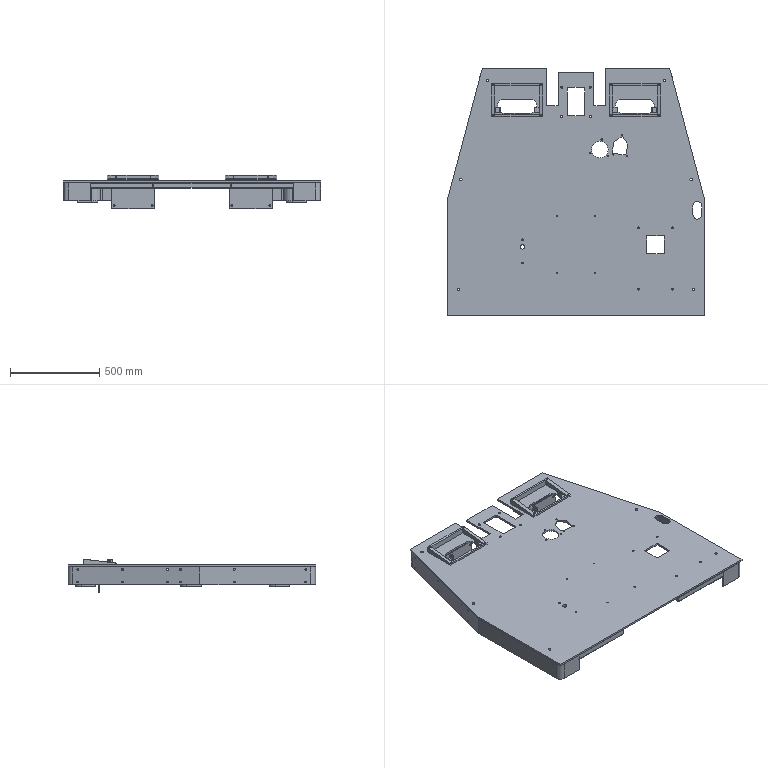Part | SolidWorks | 37 solids | 557 faces | box 1440 x 1385 x 188.942 mm | volume 24430665 mm3 | plane 295 | cylinder 238 | torus 24 | commonest cylinder face diameters 10 x76 4 x30 8 x30 68 x18 11 x16 14 x12